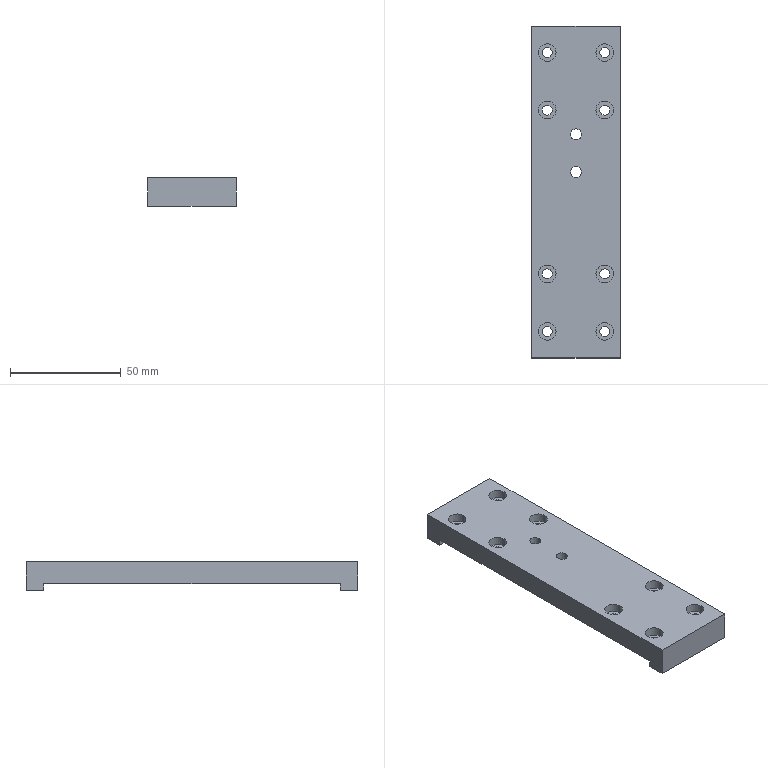Part | Creo | features CURVE 3, DATUM PLANE 3, PROTRUSION 2, COORDINATE SYSTEM 1, CUT 1 | 1 solid | 54 faces | box 40 x 150 x 13 mm | volume 59155 mm3 | cylinder 36 | plane 18 | commonest cylinder face diameters 4.5 x16 8 x16 5 x4